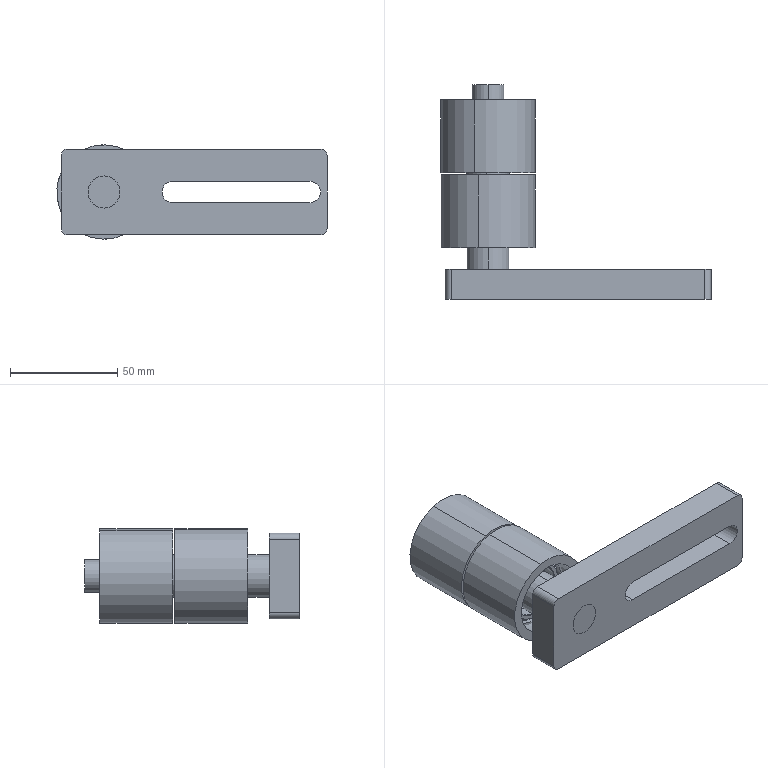Part | SolidWorks | 10 solids | 788 faces | box 126 x 100 x 44 mm | volume 132908 mm3 | spline 664 | cylinder 84 | plane 38 | cone 2 | commonest cylinder face diameters 29 x16 33 x16 15 x8 25 x8 35 x8 37 x8